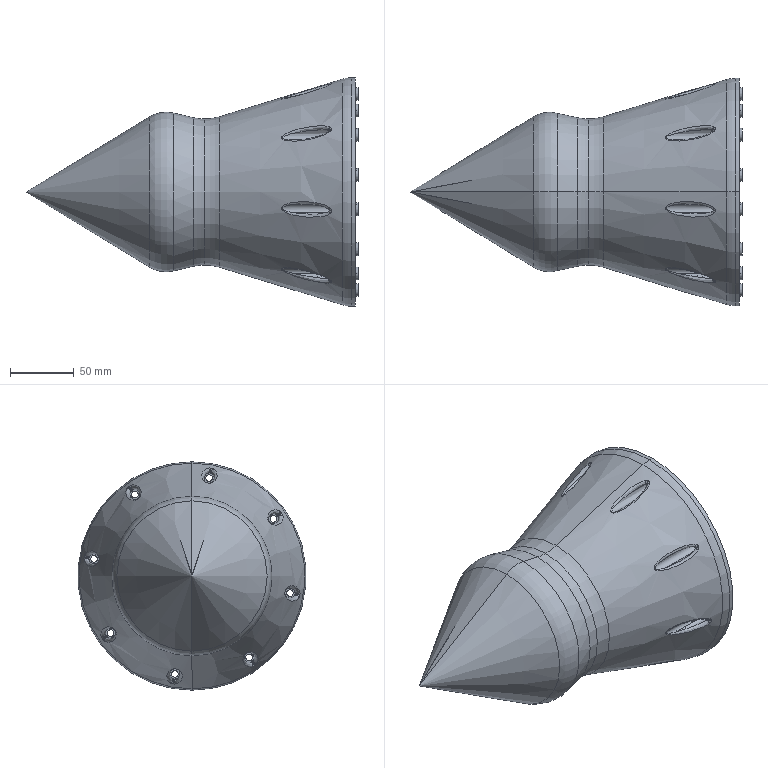Part | STEP file | Completa.sldasm-Part-22_Valor predeterminado | 1 solid | 145 faces | box 260.435 x 179.116 x 179.116 mm | volume 192197 mm3 | cylinder 52 | spline 48 | plane 17 | torus 16 | cone 12 | commonest cylinder face diameters 5.2 x16 8 x16 10 x16 175.116 x2 179.116 x2